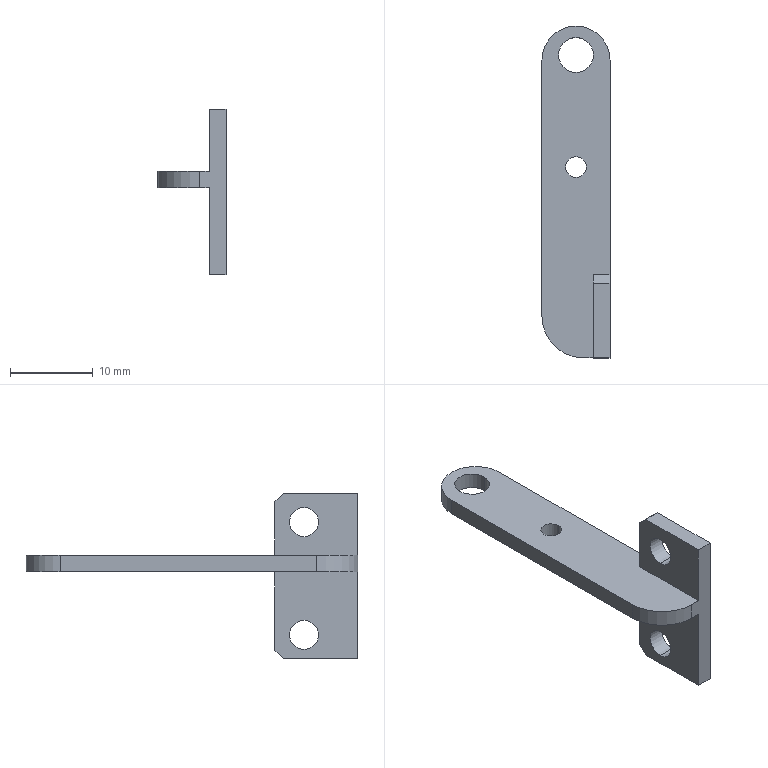Part | STEP file | 11-FG-B08111 | 1 solid | 24 faces | box 8.2 x 40 x 20 mm | volume 912.829 mm3 | plane 13 | cylinder 11 | commonest cylinder face diameters 3.5 x4 2.5 x2 4.2 x2 8.2 x2 10 x1
STEP:
#1=CARTESIAN_POINT('',(-1.25,3.,0.));
#2=VERTEX_POINT('',#1);
#3=CARTESIAN_POINT('',(1.25,3.,0.));
#4=VERTEX_POINT('',#3);
#5=CARTESIAN_POINT('',(0.,3.,0.));
#6=DIRECTION('',(0.,0.,1.));
#7=DIRECTION('',(1.,0.,0.));
#8=AXIS2_PLACEMENT_3D('',#5,#6,#7);
#9=CIRCLE('',#8,1.25);
#10=EDGE_CURVE('',#2,#4,#9,.T.);
#11=ORIENTED_EDGE('',*,*,#10,.F.);
#12=CARTESIAN_POINT('',(-1.25,3.,2.));
#13=VERTEX_POINT('',#12);
#14=CARTESIAN_POINT('',(-1.25,3.,2.));
#15=DIRECTION('',(0.,0.,1.));
#16=VECTOR('',#15,1000.);
#17=LINE('',#14,#16);
#18=EDGE_CURVE('',#2,#13,#17,.T.);
#19=ORIENTED_EDGE('',*,*,#18,.T.);
#20=CARTESIAN_POINT('',(1.25,3.,2.));
#21=VERTEX_POINT('',#20);
#22=CARTESIAN_POINT('',(0.,3.,2.));
#23=DIRECTION('',(0.,0.,1.));
#24=DIRECTION('',(1.,0.,0.));
#25=AXIS2_PLACEMENT_3D('',#22,#23,#24);
#26=CIRCLE('',#25,1.25);
#27=EDGE_CURVE('',#13,#21,#26,.T.);
#28=ORIENTED_EDGE('',*,*,#27,.T.);
#29=CARTESIAN_POINT('',(1.25,3.,2.));
#30=DIRECTION('',(0.,0.,1.));
#31=VECTOR('',#30,1000.);
#32=LINE('',#29,#31);
#33=EDGE_CURVE('',#4,#21,#32,.T.);
#34=ORIENTED_EDGE('',*,*,#33,.F.);
#35=EDGE_LOOP('',(#11,#19,#28,#34));
#36=FACE_OUTER_BOUND('',#35,.T.);
#37=CARTESIAN_POINT('',(0.,3.,2.));
#38=DIRECTION('',(0.,0.,1.));
#39=DIRECTION('',(1.,0.,0.));
#40=AXIS2_PLACEMENT_3D('',#37,#38,#39);
#41=CYLINDRICAL_SURFACE('',#40,1.25);
#42=ADVANCED_FACE('',(#36),#41,.F.);
#43=CARTESIAN_POINT('',(4.1,-13.5,-9.35));
#44=VERTEX_POINT('',#43);
#45=CARTESIAN_POINT('',(4.1,-13.5,-5.85));
#46=VERTEX_POINT('',#45);
#47=CARTESIAN_POINT('',(4.1,-13.5,-7.6));
#48=DIRECTION('',(-1.,0.,0.));
#49=DIRECTION('',(0.,-1.,0.));
#50=AXIS2_PLACEMENT_3D('',#47,#48,#49);
#51=CIRCLE('',#50,1.75);
#52=EDGE_CURVE('',#44,#46,#51,.T.);
#53=ORIENTED_EDGE('',*,*,#52,.F.);
#54=CARTESIAN_POINT('',(2.1,-13.5,-9.35));
#55=VERTEX_POINT('',#54);
#56=CARTESIAN_POINT('',(9.6,-13.5,-9.35));
#57=DIRECTION('',(-1.,0.,0.));
#58=VECTOR('',#57,1000.);
#59=LINE('',#56,#58);
#60=EDGE_CURVE('',#44,#55,#59,.T.);
#61=ORIENTED_EDGE('',*,*,#60,.T.);
#62=CARTESIAN_POINT('',(2.1,-13.5,-5.85));
#63=VERTEX_POINT('',#62);
#64=CARTESIAN_POINT('',(2.1,-13.5,-7.6));
#65=DIRECTION('',(-1.,0.,0.));
#66=DIRECTION('',(0.,0.,1.));
#67=AXIS2_PLACEMENT_3D('',#64,#65,#66);
#68=CIRCLE('',#67,1.75);
#69=EDGE_CURVE('',#55,#63,#68,.T.);
#70=ORIENTED_EDGE('',*,*,#69,.T.);
#71=CARTESIAN_POINT('',(9.6,-13.5,-5.85));
#72=DIRECTION('',(-1.,0.,0.));
#73=VECTOR('',#72,1000.);
#74=LINE('',#71,#73);
#75=EDGE_CURVE('',#46,#63,#74,.T.);
#76=ORIENTED_EDGE('',*,*,#75,.F.);
#77=EDGE_LOOP('',(#53,#61,#70,#76));
#78=FACE_OUTER_BOUND('',#77,.T.);
#79=CARTESIAN_POINT('',(9.6,-13.5,-7.6));
#80=DIRECTION('',(-1.,0.,0.));
#81=DIRECTION('',(0.,0.,1.));
#82=AXIS2_PLACEMENT_3D('',#79,#80,#81);
#83=CYLINDRICAL_SURFACE('',#82,1.75);
#84=ADVANCED_FACE('',(#78),#83,.F.);
#85=CARTESIAN_POINT('',(4.1,-13.5,4.25));
#86=VERTEX_POINT('',#85);
#87=CARTESIAN_POINT('',(4.1,-13.5,7.75));
#88=VERTEX_POINT('',#87);
#89=CARTESIAN_POINT('',(4.1,-13.5,6.));
#90=DIRECTION('',(-1.,0.,0.));
#91=DIRECTION('',(0.,-1.,0.));
#92=AXIS2_PLACEMENT_3D('',#89,#90,#91);
#93=CIRCLE('',#92,1.75);
#94=EDGE_CURVE('',#86,#88,#93,.T.);
#95=ORIENTED_EDGE('',*,*,#94,.F.);
#96=CARTESIAN_POINT('',(2.1,-13.5,4.25));
#97=VERTEX_POINT('',#96);
#98=CARTESIAN_POINT('',(9.6,-13.5,4.25));
#99=DIRECTION('',(-1.,0.,0.));
#100=VECTOR('',#99,1000.);
#101=LINE('',#98,#100);
#102=EDGE_CURVE('',#86,#97,#101,.T.);
#103=ORIENTED_EDGE('',*,*,#102,.T.);
#104=CARTESIAN_POINT('',(2.1,-13.5,7.75));
#105=VERTEX_POINT('',#104);
#106=CARTESIAN_POINT('',(2.1,-13.5,6.));
#107=DIRECTION('',(-1.,0.,0.));
#108=DIRECTION('',(0.,0.,1.));
#109=AXIS2_PLACEMENT_3D('',#106,#107,#108);
#110=CIRCLE('',#109,1.75);
#111=EDGE_CURVE('',#97,#105,#110,.T.);
#112=ORIENTED_EDGE('',*,*,#111,.T.);
#113=CARTESIAN_POINT('',(9.6,-13.5,7.75));
#114=DIRECTION('',(-1.,0.,0.));
#115=VECTOR('',#114,1000.);
#116=LINE('',#113,#115);
#117=EDGE_CURVE('',#88,#105,#116,.T.);
#118=ORIENTED_EDGE('',*,*,#117,.F.);
#119=EDGE_LOOP('',(#95,#103,#112,#118));
#120=FACE_OUTER_BOUND('',#119,.T.);
#121=CARTESIAN_POINT('',(9.6,-13.5,6.));
#122=DIRECTION('',(-1.,0.,0.));
#123=DIRECTION('',(0.,0.,1.));
#124=AXIS2_PLACEMENT_3D('',#121,#122,#123);
#125=CYLINDRICAL_SURFACE('',#124,1.75);
#126=ADVANCED_FACE('',(#120),#125,.F.);
#127=CARTESIAN_POINT('',(-2.1,16.5,0.));
#128=VERTEX_POINT('',#127);
#129=CARTESIAN_POINT('',(2.1,16.5,0.));
#130=VERTEX_POINT('',#129);
#131=CARTESIAN_POINT('',(0.,16.5,0.));
#132=DIRECTION('',(0.,0.,1.));
#133=DIRECTION('',(1.,0.,0.));
#134=AXIS2_PLACEMENT_3D('',#131,#132,#133);
#135=CIRCLE('',#134,2.1);
#136=EDGE_CURVE('',#128,#130,#135,.T.);
#137=ORIENTED_EDGE('',*,*,#136,.F.);
#138=CARTESIAN_POINT('',(-2.1,16.5,2.));
#139=VERTEX_POINT('',#138);
#140=CARTESIAN_POINT('',(-2.1,16.5,0.));
#141=DIRECTION('',(0.,0.,1.));
#142=VECTOR('',#141,1000.);
#143=LINE('',#140,#142);
#144=EDGE_CURVE('',#128,#139,#143,.T.);
#145=ORIENTED_EDGE('',*,*,#144,.T.);
#146=CARTESIAN_POINT('',(2.1,16.5,2.));
#147=VERTEX_POINT('',#146);
#148=CARTESIAN_POINT('',(0.,16.5,2.));
#149=DIRECTION('',(0.,0.,1.));
#150=DIRECTION('',(1.,0.,0.));
#151=AXIS2_PLACEMENT_3D('',#148,#149,#150);
#152=CIRCLE('',#151,2.1);
#153=EDGE_CURVE('',#139,#147,#152,.T.);
#154=ORIENTED_EDGE('',*,*,#153,.T.);
#155=CARTESIAN_POINT('',(2.1,16.5,0.));
#156=DIRECTION('',(0.,0.,1.));
#157=VECTOR('',#156,1000.);
#158=LINE('',#155,#157);
#159=EDGE_CURVE('',#130,#147,#158,.T.);
#160=ORIENTED_EDGE('',*,*,#159,.F.);
#161=EDGE_LOOP('',(#137,#145,#154,#160));
#162=FACE_OUTER_BOUND('',#161,.T.);
#163=CARTESIAN_POINT('',(0.,16.5,0.));
#164=DIRECTION('',(0.,0.,1.));
#165=DIRECTION('',(1.,0.,0.));
#166=AXIS2_PLACEMENT_3D('',#163,#164,#165);
#167=CYLINDRICAL_SURFACE('',#166,2.1);
#168=ADVANCED_FACE('',(#162),#167,.F.);
#169=CARTESIAN_POINT('',(0.,3.,0.));
#170=DIRECTION('',(0.,0.,1.));
#171=DIRECTION('',(1.,0.,0.));
#172=AXIS2_PLACEMENT_3D('',#169,#170,#171);
#173=CIRCLE('',#172,1.25);
#174=EDGE_CURVE('',#4,#2,#173,.T.);
#175=ORIENTED_EDGE('',*,*,#174,.T.);
#176=ORIENTED_EDGE('',*,*,#10,.T.);
#177=EDGE_LOOP('',(#175,#176));
#178=FACE_BOUND('',#177,.T.);
#179=CARTESIAN_POINT('',(0.,16.5,0.));
#180=DIRECTION('',(0.,0.,1.));
#181=DIRECTION('',(1.,0.,0.));
#182=AXIS2_PLACEMENT_3D('',#179,#180,#181);
#183=CIRCLE('',#182,2.1);
#184=EDGE_CURVE('',#130,#128,#183,.T.);
#185=ORIENTED_EDGE('',*,*,#184,.T.);
#186=ORIENTED_EDGE('',*,*,#136,.T.);
#187=EDGE_LOOP('',(#185,#186));
#188=FACE_BOUND('',#187,.T.);
#189=CARTESIAN_POINT('',(0.9,-20.,0.));
#190=VERTEX_POINT('',#189);
#191=CARTESIAN_POINT('',(2.1,-20.,0.));
#192=VERTEX_POINT('',#191);
#193=CARTESIAN_POINT('',(-14.1,-20.,0.));
#194=DIRECTION('',(1.,0.,0.));
#195=VECTOR('',#194,1000.);
#196=LINE('',#193,#195);
#197=EDGE_CURVE('',#190,#192,#196,.T.);
#198=ORIENTED_EDGE('',*,*,#197,.F.);
#199=CARTESIAN_POINT('',(-4.1,-15.,0.));
#200=VERTEX_POINT('',#199);
#201=CARTESIAN_POINT('',(0.9,-15.,0.));
#202=DIRECTION('',(0.,0.,-1.));
#203=DIRECTION('',(1.,0.,0.));
#204=AXIS2_PLACEMENT_3D('',#201,#202,#203);
#205=CIRCLE('',#204,5.);
#206=EDGE_CURVE('',#190,#200,#205,.T.);
#207=ORIENTED_EDGE('',*,*,#206,.T.);
#208=CARTESIAN_POINT('',(-4.1,15.9,0.));
#209=VERTEX_POINT('',#208);
#210=CARTESIAN_POINT('',(-4.1,20.,0.));
#211=DIRECTION('',(0.,1.,0.));
#212=VECTOR('',#211,1000.);
#213=LINE('',#210,#212);
#214=EDGE_CURVE('',#200,#209,#213,.T.);
#215=ORIENTED_EDGE('',*,*,#214,.T.);
#216=CARTESIAN_POINT('',(0.,20.,0.));
#217=VERTEX_POINT('',#216);
#218=CARTESIAN_POINT('',(0.,15.9,0.));
#219=DIRECTION('',(0.,0.,-1.));
#220=DIRECTION('',(1.,0.,0.));
#221=AXIS2_PLACEMENT_3D('',#218,#219,#220);
#222=CIRCLE('',#221,4.1);
#223=EDGE_CURVE('',#209,#217,#222,.T.);
#224=ORIENTED_EDGE('',*,*,#223,.T.);
#225=CARTESIAN_POINT('',(4.1,15.9,0.));
#226=VERTEX_POINT('',#225);
#227=CARTESIAN_POINT('',(0.,15.9,0.));
#228=DIRECTION('',(0.,0.,-1.));
#229=DIRECTION('',(1.,0.,0.));
#230=AXIS2_PLACEMENT_3D('',#227,#228,#229);
#231=CIRCLE('',#230,4.1);
#232=EDGE_CURVE('',#217,#226,#231,.T.);
#233=ORIENTED_EDGE('',*,*,#232,.T.);
#234=CARTESIAN_POINT('',(4.1,-10.,0.));
#235=VERTEX_POINT('',#234);
#236=CARTESIAN_POINT('',(4.1,20.,0.));
#237=DIRECTION('',(0.,-1.,0.));
#238=VECTOR('',#237,1000.);
#239=LINE('',#236,#238);
#240=EDGE_CURVE('',#226,#235,#239,.T.);
#241=ORIENTED_EDGE('',*,*,#240,.T.);
#242=CARTESIAN_POINT('',(2.1,-10.,0.));
#243=VERTEX_POINT('',#242);
#244=CARTESIAN_POINT('',(2.1,-10.,0.));
#245=DIRECTION('',(1.,0.,0.));
#246=VECTOR('',#245,1000.);
#247=LINE('',#244,#246);
#248=EDGE_CURVE('',#243,#235,#247,.T.);
#249=ORIENTED_EDGE('',*,*,#248,.F.);
#250=CARTESIAN_POINT('',(2.1,-10.,0.));
#251=DIRECTION('',(0.,1.,0.));
#252=VECTOR('',#251,1000.);
#253=LINE('',#250,#252);
#254=EDGE_CURVE('',#192,#243,#253,.T.);
#255=ORIENTED_EDGE('',*,*,#254,.F.);
#256=EDGE_LOOP('',(#198,#207,#215,#224,#233,#241,#249,#255));
#257=FACE_OUTER_BOUND('',#256,.T.);
#258=CARTESIAN_POINT('',(0.,0.,0.));
#259=DIRECTION('',(0.,0.,1.));
#260=DIRECTION('',(1.,0.,0.));
#261=AXIS2_PLACEMENT_3D('',#258,#259,#260);
#262=PLANE('',#261);
#263=ADVANCED_FACE('',(#178,#188,#257),#262,.F.);
#264=CARTESIAN_POINT('',(0.9,-20.,2.));
#265=VERTEX_POINT('',#264);
#266=CARTESIAN_POINT('',(2.1,-20.,2.));
#267=VERTEX_POINT('',#266);
#268=CARTESIAN_POINT('',(-14.1,-20.,2.));
#269=DIRECTION('',(1.,0.,0.));
#270=VECTOR('',#269,1000.);
#271=LINE('',#268,#270);
#272=EDGE_CURVE('',#265,#267,#271,.T.);
#273=ORIENTED_EDGE('',*,*,#272,.F.);
#274=CARTESIAN_POINT('',(0.9,-20.,2.));
#275=DIRECTION('',(0.,0.,-1.));
#276=VECTOR('',#275,1000.);
#277=LINE('',#274,#276);
#278=EDGE_CURVE('',#265,#190,#277,.T.);
#279=ORIENTED_EDGE('',*,*,#278,.T.);
#280=ORIENTED_EDGE('',*,*,#197,.T.);
#281=CARTESIAN_POINT('',(2.1,-20.,-10.5));
#282=VERTEX_POINT('',#281);
#283=CARTESIAN_POINT('',(2.1,-20.,-10.5));
#284=DIRECTION('',(0.,0.,1.));
#285=VECTOR('',#284,1000.);
#286=LINE('',#283,#285);
#287=EDGE_CURVE('',#282,#192,#286,.T.);
#288=ORIENTED_EDGE('',*,*,#287,.F.);
#289=CARTESIAN_POINT('',(4.1,-20.,-10.5));
#290=VERTEX_POINT('',#289);
#291=CARTESIAN_POINT('',(2.1,-20.,-10.5));
#292=DIRECTION('',(-1.,0.,0.));
#293=VECTOR('',#292,1000.);
#294=LINE('',#291,#293);
#295=EDGE_CURVE('',#290,#282,#294,.T.);
#296=ORIENTED_EDGE('',*,*,#295,.F.);
#297=CARTESIAN_POINT('',(4.1,-20.,9.5));
#298=VERTEX_POINT('',#297);
#299=CARTESIAN_POINT('',(4.1,-20.,-22.));
#300=DIRECTION('',(0.,0.,1.));
#301=VECTOR('',#300,1000.);
#302=LINE('',#299,#301);
#303=EDGE_CURVE('',#290,#298,#302,.T.);
#304=ORIENTED_EDGE('',*,*,#303,.T.);
#305=CARTESIAN_POINT('',(2.1,-20.,9.5));
#306=VERTEX_POINT('',#305);
#307=CARTESIAN_POINT('',(4.1,-20.,9.5));
#308=DIRECTION('',(1.,0.,0.));
#309=VECTOR('',#308,1000.);
#310=LINE('',#307,#309);
#311=EDGE_CURVE('',#306,#298,#310,.T.);
#312=ORIENTED_EDGE('',*,*,#311,.F.);
#313=CARTESIAN_POINT('',(2.1,-20.,9.5));
#314=DIRECTION('',(0.,0.,-1.));
#315=VECTOR('',#314,1000.);
#316=LINE('',#313,#315);
#317=EDGE_CURVE('',#306,#267,#316,.T.);
#318=ORIENTED_EDGE('',*,*,#317,.T.);
#319=EDGE_LOOP('',(#273,#279,#280,#288,#296,#304,#312,#318));
#320=FACE_OUTER_BOUND('',#319,.T.);
#321=CARTESIAN_POINT('',(-14.1,-20.,2.));
#322=DIRECTION('',(0.,1.,0.));
#323=DIRECTION('',(0.,0.,1.));
#324=AXIS2_PLACEMENT_3D('',#321,#322,#323);
#325=PLANE('',#324);
#326=ADVANCED_FACE('',(#320),#325,.F.);
#327=CARTESIAN_POINT('',(0.,3.,2.));
#328=DIRECTION('',(0.,0.,1.));
#329=DIRECTION('',(1.,0.,0.));
#330=AXIS2_PLACEMENT_3D('',#327,#328,#329);
#331=CIRCLE('',#330,1.25);
#332=EDGE_CURVE('',#21,#13,#331,.T.);
#333=ORIENTED_EDGE('',*,*,#332,.F.);
#334=ORIENTED_EDGE('',*,*,#27,.F.);
#335=EDGE_LOOP('',(#333,#334));
#336=FACE_BOUND('',#335,.T.);
#337=CARTESIAN_POINT('',(-4.1,-15.,2.));
#338=VERTEX_POINT('',#337);
#339=CARTESIAN_POINT('',(-4.1,15.9,2.));
#340=VERTEX_POINT('',#339);
#341=CARTESIAN_POINT('',(-4.1,20.,2.));
#342=DIRECTION('',(0.,1.,0.));
#343=VECTOR('',#342,1000.);
#344=LINE('',#341,#343);
#345=EDGE_CURVE('',#338,#340,#344,.T.);
#346=ORIENTED_EDGE('',*,*,#345,.F.);
#347=CARTESIAN_POINT('',(0.9,-15.,2.));
#348=DIRECTION('',(0.,0.,1.));
#349=DIRECTION('',(1.,0.,0.));
#350=AXIS2_PLACEMENT_3D('',#347,#348,#349);
#351=CIRCLE('',#350,5.);
#352=EDGE_CURVE('',#338,#265,#351,.T.);
#353=ORIENTED_EDGE('',*,*,#352,.T.);
#354=ORIENTED_EDGE('',*,*,#272,.T.);
#355=CARTESIAN_POINT('',(2.1,-10.,2.));
#356=VERTEX_POINT('',#355);
#357=CARTESIAN_POINT('',(2.1,-20.,2.));
#358=DIRECTION('',(0.,-1.,0.));
#359=VECTOR('',#358,1000.);
#360=LINE('',#357,#359);
#361=EDGE_CURVE('',#356,#267,#360,.T.);
#362=ORIENTED_EDGE('',*,*,#361,.F.);
#363=CARTESIAN_POINT('',(4.1,-10.,2.));
#364=VERTEX_POINT('',#363);
#365=CARTESIAN_POINT('',(4.1,-10.,2.));
#366=DIRECTION('',(-1.,0.,0.));
#367=VECTOR('',#366,1000.);
#368=LINE('',#365,#367);
#369=EDGE_CURVE('',#364,#356,#368,.T.);
#370=ORIENTED_EDGE('',*,*,#369,.F.);
#371=CARTESIAN_POINT('',(4.1,15.9,2.));
#372=VERTEX_POINT('',#371);
#373=CARTESIAN_POINT('',(4.1,20.,2.));
#374=DIRECTION('',(0.,-1.,0.));
#375=VECTOR('',#374,1000.);
#376=LINE('',#373,#375);
#377=EDGE_CURVE('',#372,#364,#376,.T.);
#378=ORIENTED_EDGE('',*,*,#377,.F.);
#379=CARTESIAN_POINT('',(0.,20.,2.));
#380=VERTEX_POINT('',#379);
#381=CARTESIAN_POINT('',(0.,15.9,2.));
#382=DIRECTION('',(0.,0.,1.));
#383=DIRECTION('',(1.,0.,0.));
#384=AXIS2_PLACEMENT_3D('',#381,#382,#383);
#385=CIRCLE('',#384,4.1);
#386=EDGE_CURVE('',#372,#380,#385,.T.);
#387=ORIENTED_EDGE('',*,*,#386,.T.);
#388=CARTESIAN_POINT('',(0.,15.9,2.));
#389=DIRECTION('',(0.,0.,1.));
#390=DIRECTION('',(1.,0.,0.));
#391=AXIS2_PLACEMENT_3D('',#388,#389,#390);
#392=CIRCLE('',#391,4.1);
#393=EDGE_CURVE('',#380,#340,#392,.T.);
#394=ORIENTED_EDGE('',*,*,#393,.T.);
#395=EDGE_LOOP('',(#346,#353,#354,#362,#370,#378,#387,#394));
#396=FACE_OUTER_BOUND('',#395,.T.);
#397=CARTESIAN_POINT('',(0.,16.5,2.));
#398=DIRECTION('',(0.,0.,1.));
#399=DIRECTION('',(1.,0.,0.));
#400=AXIS2_PLACEMENT_3D('',#397,#398,#399);
#401=CIRCLE('',#400,2.1);
#402=EDGE_CURVE('',#147,#139,#401,.T.);
#403=ORIENTED_EDGE('',*,*,#402,.F.);
#404=ORIENTED_EDGE('',*,*,#153,.F.);
#405=EDGE_LOOP('',(#403,#404));
#406=FACE_BOUND('',#405,.T.);
#407=CARTESIAN_POINT('',(0.,0.,2.));
#408=DIRECTION('',(0.,0.,1.));
#409=DIRECTION('',(1.,0.,0.));
#410=AXIS2_PLACEMENT_3D('',#407,#408,#409);
#411=PLANE('',#410);
#412=ADVANCED_FACE('',(#336,#396,#406),#411,.T.);
#413=ORIENTED_EDGE('',*,*,#214,.F.);
#414=CARTESIAN_POINT('',(-4.1,-15.,0.));
#415=DIRECTION('',(0.,0.,1.));
#416=VECTOR('',#415,1000.);
#417=LINE('',#414,#416);
#418=EDGE_CURVE('',#200,#338,#417,.T.);
#419=ORIENTED_EDGE('',*,*,#418,.T.);
#420=ORIENTED_EDGE('',*,*,#345,.T.);
#421=CARTESIAN_POINT('',(-4.1,15.9,0.));
#422=DIRECTION('',(0.,0.,-1.));
#423=VECTOR('',#422,1000.);
#424=LINE('',#421,#423);
#425=EDGE_CURVE('',#340,#209,#424,.T.);
#426=ORIENTED_EDGE('',*,*,#425,.T.);
#427=EDGE_LOOP('',(#413,#419,#420,#426));
#428=FACE_OUTER_BOUND('',#427,.T.);
#429=CARTESIAN_POINT('',(-4.1,20.,0.));
#430=DIRECTION('',(1.,0.,0.));
#431=DIRECTION('',(0.,1.,0.));
#432=AXIS2_PLACEMENT_3D('',#429,#430,#431);
#433=PLANE('',#432);
#434=ADVANCED_FACE('',(#428),#433,.F.);
#435=CARTESIAN_POINT('',(4.1,-13.5,-7.6));
#436=DIRECTION('',(-1.,0.,0.));
#437=DIRECTION('',(0.,-1.,0.));
#438=AXIS2_PLACEMENT_3D('',#435,#436,#437);
#439=CIRCLE('',#438,1.75);
#440=EDGE_CURVE('',#46,#44,#439,.T.);
#441=ORIENTED_EDGE('',*,*,#440,.T.);
#442=ORIENTED_EDGE('',*,*,#52,.T.);
#443=EDGE_LOOP('',(#441,#442));
#444=FACE_BOUND('',#443,.T.);
#445=CARTESIAN_POINT('',(4.1,-13.5,6.));
#446=DIRECTION('',(-1.,0.,0.));
#447=DIRECTION('',(0.,-1.,0.));
#448=AXIS2_PLACEMENT_3D('',#445,#446,#447);
#449=CIRCLE('',#448,1.75);
#450=EDGE_CURVE('',#88,#86,#449,.T.);
#451=ORIENTED_EDGE('',*,*,#450,.T.);
#452=ORIENTED_EDGE('',*,*,#94,.T.);
#453=EDGE_LOOP('',(#451,#452));
#454=FACE_BOUND('',#453,.T.);
#455=CARTESIAN_POINT('',(4.1,-10.,8.5));
#456=VERTEX_POINT('',#455);
#457=CARTESIAN_POINT('',(4.1,-10.,9.5));
#458=DIRECTION('',(0.,0.,-1.));
#459=VECTOR('',#458,1000.);
#460=LINE('',#457,#459);
#461=EDGE_CURVE('',#456,#364,#460,.T.);
#462=ORIENTED_EDGE('',*,*,#461,.F.);
#463=CARTESIAN_POINT('',(4.1,-11.,9.5));
#464=VERTEX_POINT('',#463);
#465=CARTESIAN_POINT('',(4.1,-11.,9.5));
#466=DIRECTION('',(0.,-0.7071,0.7071));
#467=VECTOR('',#466,1000.);
#468=LINE('',#465,#467);
#469=EDGE_CURVE('',#456,#464,#468,.T.);
#470=ORIENTED_EDGE('',*,*,#469,.T.);
#471=CARTESIAN_POINT('',(4.1,-20.,9.5));
#472=DIRECTION('',(0.,1.,0.));
#473=VECTOR('',#472,1000.);
#474=LINE('',#471,#473);
#475=EDGE_CURVE('',#298,#464,#474,.T.);
#476=ORIENTED_EDGE('',*,*,#475,.F.);
#477=ORIENTED_EDGE('',*,*,#303,.F.);
#478=CARTESIAN_POINT('',(4.1,-11.,-10.5));
#479=VERTEX_POINT('',#478);
#480=CARTESIAN_POINT('',(4.1,-10.,-10.5));
#481=DIRECTION('',(0.,-1.,0.));
#482=VECTOR('',#481,1000.);
#483=LINE('',#480,#482);
#484=EDGE_CURVE('',#479,#290,#483,.T.);
#485=ORIENTED_EDGE('',*,*,#484,.F.);
#486=CARTESIAN_POINT('',(4.1,-10.,-9.5));
#487=VERTEX_POINT('',#486);
#488=CARTESIAN_POINT('',(4.1,-11.,-10.5));
#489=DIRECTION('',(0.,0.7071,0.7071));
#490=VECTOR('',#489,1000.);
#491=LINE('',#488,#490);
#492=EDGE_CURVE('',#479,#487,#491,.T.);
#493=ORIENTED_EDGE('',*,*,#492,.T.);
#494=CARTESIAN_POINT('',(4.1,-10.,-10.5));
#495=DIRECTION('',(0.,0.,1.));
#496=VECTOR('',#495,1000.);
#497=LINE('',#494,#496);
#498=EDGE_CURVE('',#487,#235,#497,.T.);
#499=ORIENTED_EDGE('',*,*,#498,.T.);
#500=ORIENTED_EDGE('',*,*,#240,.F.);
#501=CARTESIAN_POINT('',(4.1,15.9,0.));
#502=DIRECTION('',(0.,0.,1.));
#503=VECTOR('',#502,1000.);
#504=LINE('',#501,#503);
#505=EDGE_CURVE('',#226,#372,#504,.T.);
#506=ORIENTED_EDGE('',*,*,#505,.T.);
#507=ORIENTED_EDGE('',*,*,#377,.T.);
#508=EDGE_LOOP('',(#462,#470,#476,#477,#485,#493,#499,#500,#506,#507));
#509=FACE_OUTER_BOUND('',#508,.T.);
#510=CARTESIAN_POINT('',(4.1,20.,0.));
#511=DIRECTION('',(-1.,0.,0.));
#512=DIRECTION('',(0.,-1.,0.));
#513=AXIS2_PLACEMENT_3D('',#510,#511,#512);
#514=PLANE('',#513);
#515=ADVANCED_FACE('',(#444,#454,#509),#514,.F.);
#516=ORIENTED_EDGE('',*,*,#144,.F.);
#517=ORIENTED_EDGE('',*,*,#184,.F.);
#518=ORIENTED_EDGE('',*,*,#159,.T.);
#519=ORIENTED_EDGE('',*,*,#402,.T.);
#520=EDGE_LOOP('',(#516,#517,#518,#519));
#521=FACE_OUTER_BOUND('',#520,.T.);
#522=CARTESIAN_POINT('',(0.,16.5,0.));
#523=DIRECTION('',(0.,0.,1.));
#524=DIRECTION('',(1.,0.,0.));
#525=AXIS2_PLACEMENT_3D('',#522,#523,#524);
#526=CYLINDRICAL_SURFACE('',#525,2.1);
#527=ADVANCED_FACE('',(#521),#526,.F.);
#528=CARTESIAN_POINT('',(0.,20.,2.));
#529=DIRECTION('',(0.,0.,1.));
#530=VECTOR('',#529,1000.);
#531=LINE('',#528,#530);
#532=EDGE_CURVE('',#217,#380,#531,.T.);
#533=ORIENTED_EDGE('',*,*,#532,.F.);
#534=ORIENTED_EDGE('',*,*,#223,.F.);
#535=ORIENTED_EDGE('',*,*,#425,.F.);
#536=ORIENTED_EDGE('',*,*,#393,.F.);
#537=EDGE_LOOP('',(#533,#534,#535,#536));
#538=FACE_OUTER_BOUND('',#537,.T.);
#539=CARTESIAN_POINT('',(0.,15.9,2.));
#540=DIRECTION('',(0.,0.,1.));
#541=DIRECTION('',(1.,0.,0.));
#542=AXIS2_PLACEMENT_3D('',#539,#540,#541);
#543=CYLINDRICAL_SURFACE('',#542,4.1);
#544=ADVANCED_FACE('',(#538),#543,.T.);
#545=ORIENTED_EDGE('',*,*,#232,.F.);
#546=ORIENTED_EDGE('',*,*,#532,.T.);
#547=ORIENTED_EDGE('',*,*,#386,.F.);
#548=ORIENTED_EDGE('',*,*,#505,.F.);
#549=EDGE_LOOP('',(#545,#546,#547,#548));
#550=FACE_OUTER_BOUND('',#549,.T.);
#551=CARTESIAN_POINT('',(0.,15.9,0.));
#552=DIRECTION('',(0.,0.,1.));
#553=DIRECTION('',(1.,0.,0.));
#554=AXIS2_PLACEMENT_3D('',#551,#552,#553);
#555=CYLINDRICAL_SURFACE('',#554,4.1);
#556=ADVANCED_FACE('',(#550),#555,.T.);
#557=CARTESIAN_POINT('',(2.1,-10.,8.5));
#558=VERTEX_POINT('',#557);
#559=CARTESIAN_POINT('',(2.1,-10.,9.5));
#560=DIRECTION('',(0.,0.,-1.));
#561=VECTOR('',#560,1000.);
#562=LINE('',#559,#561);
#563=EDGE_CURVE('',#558,#356,#562,.T.);
#564=ORIENTED_EDGE('',*,*,#563,.F.);
#565=CARTESIAN_POINT('',(4.1,-10.,8.5));
#566=DIRECTION('',(1.,0.,0.));
#567=VECTOR('',#566,1000.);
#568=LINE('',#565,#567);
#569=EDGE_CURVE('',#558,#456,#568,.T.);
#570=ORIENTED_EDGE('',*,*,#569,.T.);
#571=ORIENTED_EDGE('',*,*,#461,.T.);
#572=ORIENTED_EDGE('',*,*,#369,.T.);
#573=EDGE_LOOP('',(#564,#570,#571,#572));
#574=FACE_OUTER_BOUND('',#573,.T.);
#575=CARTESIAN_POINT('',(4.1,-10.,9.5));
#576=DIRECTION('',(0.,-1.,0.));
#577=DIRECTION('',(1.,0.,0.));
#578=AXIS2_PLACEMENT_3D('',#575,#576,#577);
#579=PLANE('',#578);
#580=ADVANCED_FACE('',(#574),#579,.F.);
#581=CARTESIAN_POINT('',(2.1,-13.5,6.));
#582=DIRECTION('',(-1.,0.,0.));
#583=DIRECTION('',(0.,0.,1.));
#584=AXIS2_PLACEMENT_3D('',#581,#582,#583);
#585=CIRCLE('',#584,1.75);
#586=EDGE_CURVE('',#105,#97,#585,.T.);
#587=ORIENTED_EDGE('',*,*,#586,.F.);
#588=ORIENTED_EDGE('',*,*,#111,.F.);
#589=EDGE_LOOP('',(#587,#588));
#590=FACE_BOUND('',#589,.T.);
#591=CARTESIAN_POINT('',(2.1,-11.,9.5));
#592=VERTEX_POINT('',#591);
#593=CARTESIAN_POINT('',(2.1,-20.,9.5));
#594=DIRECTION('',(0.,-1.,0.));
#595=VECTOR('',#594,1000.);
#596=LINE('',#593,#595);
#597=EDGE_CURVE('',#592,#306,#596,.T.);
#598=ORIENTED_EDGE('',*,*,#597,.F.);
#599=CARTESIAN_POINT('',(2.1,-11.,9.5));
#600=DIRECTION('',(0.,0.7071,-0.7071));
#601=VECTOR('',#600,1000.);
#602=LINE('',#599,#601);
#603=EDGE_CURVE('',#592,#558,#602,.T.);
#604=ORIENTED_EDGE('',*,*,#603,.T.);
#605=ORIENTED_EDGE('',*,*,#563,.T.);
#606=ORIENTED_EDGE('',*,*,#361,.T.);
#607=ORIENTED_EDGE('',*,*,#317,.F.);
#608=EDGE_LOOP('',(#598,#604,#605,#606,#607));
#609=FACE_OUTER_BOUND('',#608,.T.);
#610=CARTESIAN_POINT('',(2.1,-20.,9.5));
#611=DIRECTION('',(1.,0.,0.));
#612=DIRECTION('',(0.,0.,-1.));
#613=AXIS2_PLACEMENT_3D('',#610,#611,#612);
#614=PLANE('',#613);
#615=ADVANCED_FACE('',(#590,#609),#614,.F.);
#616=ORIENTED_EDGE('',*,*,#475,.T.);
#617=CARTESIAN_POINT('',(2.1,-11.,9.5));
#618=DIRECTION('',(-1.,0.,0.));
#619=VECTOR('',#618,1000.);
#620=LINE('',#617,#619);
#621=EDGE_CURVE('',#464,#592,#620,.T.);
#622=ORIENTED_EDGE('',*,*,#621,.T.);
#623=ORIENTED_EDGE('',*,*,#597,.T.);
#624=ORIENTED_EDGE('',*,*,#311,.T.);
#625=EDGE_LOOP('',(#616,#622,#623,#624));
#626=FACE_OUTER_BOUND('',#625,.T.);
#627=CARTESIAN_POINT('',(0.,0.,9.5));
#628=DIRECTION('',(0.,0.,1.));
#629=DIRECTION('',(1.,0.,0.));
#630=AXIS2_PLACEMENT_3D('',#627,#628,#629);
#631=PLANE('',#630);
#632=ADVANCED_FACE('',(#626),#631,.T.);
#633=CARTESIAN_POINT('',(2.1,-13.5,-7.6));
#634=DIRECTION('',(-1.,0.,0.));
#635=DIRECTION('',(0.,0.,1.));
#636=AXIS2_PLACEMENT_3D('',#633,#634,#635);
#637=CIRCLE('',#636,1.75);
#638=EDGE_CURVE('',#63,#55,#637,.T.);
#639=ORIENTED_EDGE('',*,*,#638,.F.);
#640=ORIENTED_EDGE('',*,*,#69,.F.);
#641=EDGE_LOOP('',(#639,#640));
#642=FACE_BOUND('',#641,.T.);
#643=CARTESIAN_POINT('',(2.1,-10.,-9.5));
#644=VERTEX_POINT('',#643);
#645=CARTESIAN_POINT('',(2.1,-10.,-10.5));
#646=DIRECTION('',(0.,0.,1.));
#647=VECTOR('',#646,1000.);
#648=LINE('',#645,#647);
#649=EDGE_CURVE('',#644,#243,#648,.T.);
#650=ORIENTED_EDGE('',*,*,#649,.F.);
#651=CARTESIAN_POINT('',(2.1,-11.,-10.5));
#652=VERTEX_POINT('',#651);
#653=CARTESIAN_POINT('',(2.1,-11.,-10.5));
#654=DIRECTION('',(0.,-0.7071,-0.7071));
#655=VECTOR('',#654,1000.);
#656=LINE('',#653,#655);
#657=EDGE_CURVE('',#644,#652,#656,.T.);
#658=ORIENTED_EDGE('',*,*,#657,.T.);
#659=CARTESIAN_POINT('',(2.1,-10.,-10.5));
#660=DIRECTION('',(0.,1.,0.));
#661=VECTOR('',#660,1000.);
#662=LINE('',#659,#661);
#663=EDGE_CURVE('',#282,#652,#662,.T.);
#664=ORIENTED_EDGE('',*,*,#663,.F.);
#665=ORIENTED_EDGE('',*,*,#287,.T.);
#666=ORIENTED_EDGE('',*,*,#254,.T.);
#667=EDGE_LOOP('',(#650,#658,#664,#665,#666));
#668=FACE_OUTER_BOUND('',#667,.T.);
#669=CARTESIAN_POINT('',(2.1,-10.,-10.5));
#670=DIRECTION('',(1.,0.,0.));
#671=DIRECTION('',(0.,0.,-1.));
#672=AXIS2_PLACEMENT_3D('',#669,#670,#671);
#673=PLANE('',#672);
#674=ADVANCED_FACE('',(#642,#668),#673,.F.);
#675=ORIENTED_EDGE('',*,*,#498,.F.);
#676=CARTESIAN_POINT('',(2.1,-10.,-9.5));
#677=DIRECTION('',(-1.,0.,0.));
#678=VECTOR('',#677,1000.);
#679=LINE('',#676,#678);
#680=EDGE_CURVE('',#487,#644,#679,.T.);
#681=ORIENTED_EDGE('',*,*,#680,.T.);
#682=ORIENTED_EDGE('',*,*,#649,.T.);
#683=ORIENTED_EDGE('',*,*,#248,.T.);
#684=EDGE_LOOP('',(#675,#681,#682,#683));
#685=FACE_OUTER_BOUND('',#684,.T.);
#686=CARTESIAN_POINT('',(2.1,-10.,-10.5));
#687=DIRECTION('',(0.,-1.,0.));
#688=DIRECTION('',(0.,0.,-1.));
#689=AXIS2_PLACEMENT_3D('',#686,#687,#688);
#690=PLANE('',#689);
#691=ADVANCED_FACE('',(#685),#690,.F.);
#692=ORIENTED_EDGE('',*,*,#663,.T.);
#693=CARTESIAN_POINT('',(0.,-11.,-10.5));
#694=DIRECTION('',(1.,0.,0.));
#695=VECTOR('',#694,1000.);
#696=LINE('',#693,#695);
#697=EDGE_CURVE('',#652,#479,#696,.T.);
#698=ORIENTED_EDGE('',*,*,#697,.T.);
#699=ORIENTED_EDGE('',*,*,#484,.T.);
#700=ORIENTED_EDGE('',*,*,#295,.T.);
#701=EDGE_LOOP('',(#692,#698,#699,#700));
#702=FACE_OUTER_BOUND('',#701,.T.);
#703=CARTESIAN_POINT('',(0.,0.,-10.5));
#704=DIRECTION('',(0.,0.,1.));
#705=DIRECTION('',(1.,0.,0.));
#706=AXIS2_PLACEMENT_3D('',#703,#704,#705);
#707=PLANE('',#706);
#708=ADVANCED_FACE('',(#702),#707,.F.);
#709=ORIENTED_EDGE('',*,*,#102,.F.);
#710=ORIENTED_EDGE('',*,*,#450,.F.);
#711=ORIENTED_EDGE('',*,*,#117,.T.);
#712=ORIENTED_EDGE('',*,*,#586,.T.);
#713=EDGE_LOOP('',(#709,#710,#711,#712));
#714=FACE_OUTER_BOUND('',#713,.T.);
#715=CARTESIAN_POINT('',(9.6,-13.5,6.));
#716=DIRECTION('',(-1.,0.,0.));
#717=DIRECTION('',(0.,0.,1.));
#718=AXIS2_PLACEMENT_3D('',#715,#716,#717);
#719=CYLINDRICAL_SURFACE('',#718,1.75);
#720=ADVANCED_FACE('',(#714),#719,.F.);
#721=ORIENTED_EDGE('',*,*,#60,.F.);
#722=ORIENTED_EDGE('',*,*,#440,.F.);
#723=ORIENTED_EDGE('',*,*,#75,.T.);
#724=ORIENTED_EDGE('',*,*,#638,.T.);
#725=EDGE_LOOP('',(#721,#722,#723,#724));
#726=FACE_OUTER_BOUND('',#725,.T.);
#727=CARTESIAN_POINT('',(9.6,-13.5,-7.6));
#728=DIRECTION('',(-1.,0.,0.));
#729=DIRECTION('',(0.,0.,1.));
#730=AXIS2_PLACEMENT_3D('',#727,#728,#729);
#731=CYLINDRICAL_SURFACE('',#730,1.75);
#732=ADVANCED_FACE('',(#726),#731,.F.);
#733=ORIENTED_EDGE('',*,*,#469,.F.);
#734=ORIENTED_EDGE('',*,*,#569,.F.);
#735=ORIENTED_EDGE('',*,*,#603,.F.);
#736=ORIENTED_EDGE('',*,*,#621,.F.);
#737=EDGE_LOOP('',(#733,#734,#735,#736));
#738=FACE_OUTER_BOUND('',#737,.T.);
#739=CARTESIAN_POINT('',(0.,-11.,9.5));
#740=DIRECTION('',(0.,0.7071,0.7071));
#741=DIRECTION('',(1.,0.,0.));
#742=AXIS2_PLACEMENT_3D('',#739,#740,#741);
#743=PLANE('',#742);
#744=ADVANCED_FACE('',(#738),#743,.T.);
#745=ORIENTED_EDGE('',*,*,#657,.F.);
#746=ORIENTED_EDGE('',*,*,#680,.F.);
#747=ORIENTED_EDGE('',*,*,#492,.F.);
#748=ORIENTED_EDGE('',*,*,#697,.F.);
#749=EDGE_LOOP('',(#745,#746,#747,#748));
#750=FACE_OUTER_BOUND('',#749,.T.);
#751=CARTESIAN_POINT('',(0.,-11.,-10.5));
#752=DIRECTION('',(0.,-0.7071,0.7071));
#753=DIRECTION('',(1.,0.,0.));
#754=AXIS2_PLACEMENT_3D('',#751,#752,#753);
#755=PLANE('',#754);
#756=ADVANCED_FACE('',(#750),#755,.F.);
#757=ORIENTED_EDGE('',*,*,#18,.F.);
#758=ORIENTED_EDGE('',*,*,#174,.F.);
#759=ORIENTED_EDGE('',*,*,#33,.T.);
#760=ORIENTED_EDGE('',*,*,#332,.T.);
#761=EDGE_LOOP('',(#757,#758,#759,#760));
#762=FACE_OUTER_BOUND('',#761,.T.);
#763=CARTESIAN_POINT('',(0.,3.,2.));
#764=DIRECTION('',(0.,0.,1.));
#765=DIRECTION('',(1.,0.,0.));
#766=AXIS2_PLACEMENT_3D('',#763,#764,#765);
#767=CYLINDRICAL_SURFACE('',#766,1.25);
#768=ADVANCED_FACE('',(#762),#767,.F.);
#769=ORIENTED_EDGE('',*,*,#206,.F.);
#770=ORIENTED_EDGE('',*,*,#278,.F.);
#771=ORIENTED_EDGE('',*,*,#352,.F.);
#772=ORIENTED_EDGE('',*,*,#418,.F.);
#773=EDGE_LOOP('',(#769,#770,#771,#772));
#774=FACE_OUTER_BOUND('',#773,.T.);
#775=CARTESIAN_POINT('',(0.9,-15.,0.));
#776=DIRECTION('',(0.,0.,1.));
#777=DIRECTION('',(1.,0.,0.));
#778=AXIS2_PLACEMENT_3D('',#775,#776,#777);
#779=CYLINDRICAL_SURFACE('',#778,5.);
#780=ADVANCED_FACE('',(#774),#779,.T.);
#781=CLOSED_SHELL('',(#42,#84,#126,#168,#263,#326,#412,#434,#515,#527,#544,#556,#580,#615,#632,#674,#691,#708,#720,#732,#744,#756,#768,#780));
#782=MANIFOLD_SOLID_BREP('',#781);
#783=CARTESIAN_POINT('',(0.,0.,0.));
#784=DIRECTION('',(0.,0.,1.));
#785=DIRECTION('',(1.,0.,0.));
#786=AXIS2_PLACEMENT_3D('',#783,#784,#785);
#787=(LENGTH_UNIT()NAMED_UNIT(*)SI_UNIT(.MILLI.,.METRE.));
#788=UNCERTAINTY_MEASURE_WITH_UNIT(LENGTH_MEASURE(0.00001),#787,'','');
#789=(NAMED_UNIT(*)PLANE_ANGLE_UNIT()SI_UNIT($,.RADIAN.));
#790=(NAMED_UNIT(*)SI_UNIT($,.STERADIAN.)SOLID_ANGLE_UNIT());
#791=(GEOMETRIC_REPRESENTATION_CONTEXT(3)GLOBAL_UNCERTAINTY_ASSIGNED_CONTEXT((#788))GLOBAL_UNIT_ASSIGNED_CONTEXT((#787,#789,#790))REPRESENTATION_CONTEXT('',''));
#792=ADVANCED_BREP_SHAPE_REPRESENTATION('',(#782,#786),#791);